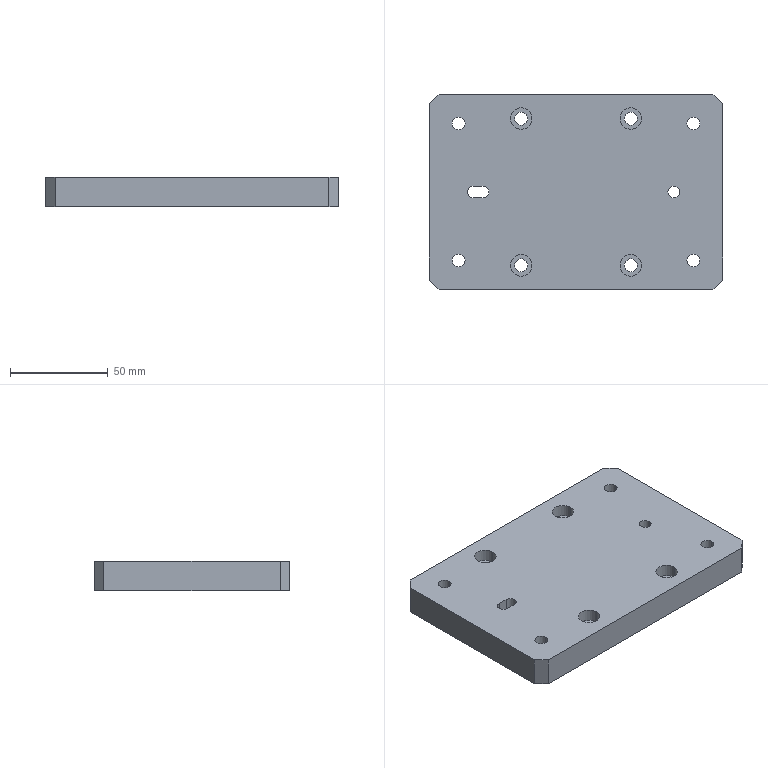Part | SolidWorks | features HoleWzd 3, Chamfer 1, Cut 1, Extrusion 1 | 1 solid | 57 faces | box 150 x 100 x 15 mm | volume 215343 mm3 | cylinder 37 | plane 20 | commonest cylinder face diameters 6.6 x16 11 x16 6 x5